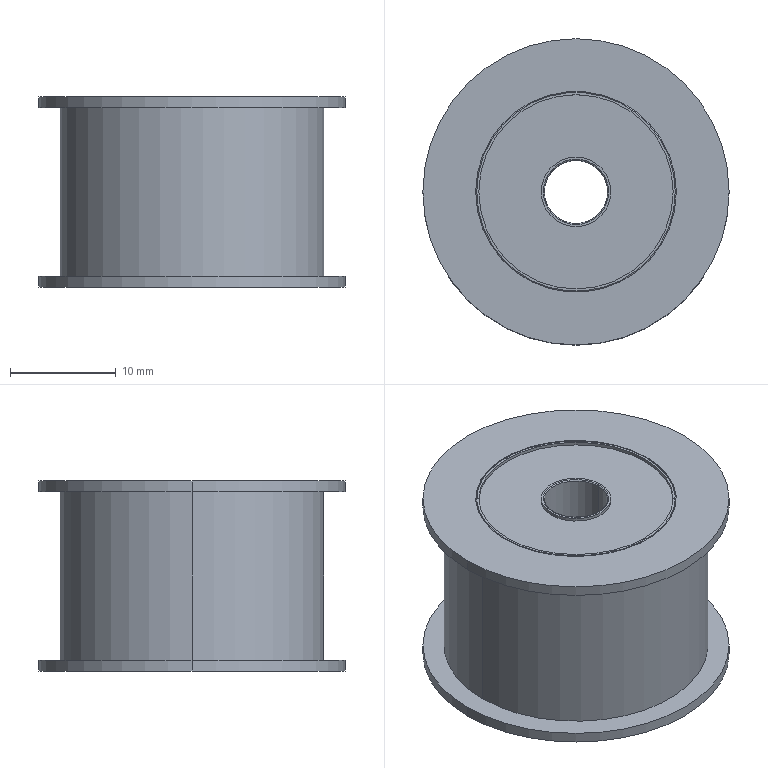Part | SolidWorks | features BaseBody 1 | 1 solid | 63 faces | box 29 x 29 x 18 mm | volume 7351 mm3 | cylinder 34 | plane 17 | torus 12 | commonest cylinder face diameters 6.6 x8 18.4 x8 19 x6 6 x4 29 x4 16 x2